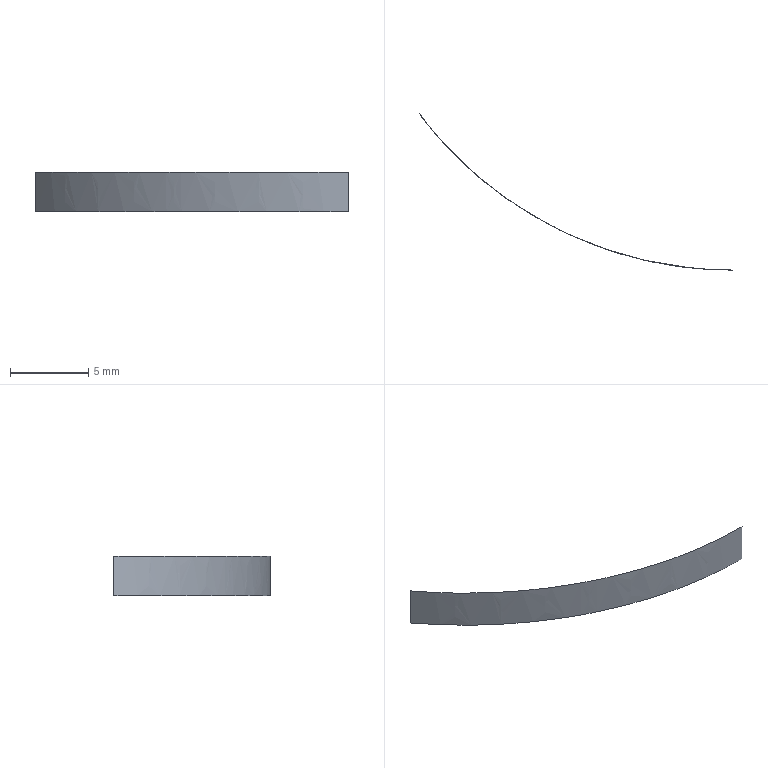Part | STEP file | lll_id374_x_t | 1 solid | 2 faces | box 19.966 x 9.955 x 2.5 mm | volume 0.1857 mm3 | other 1 | cylinder 1 | commonest cylinder face diameters 50 x1